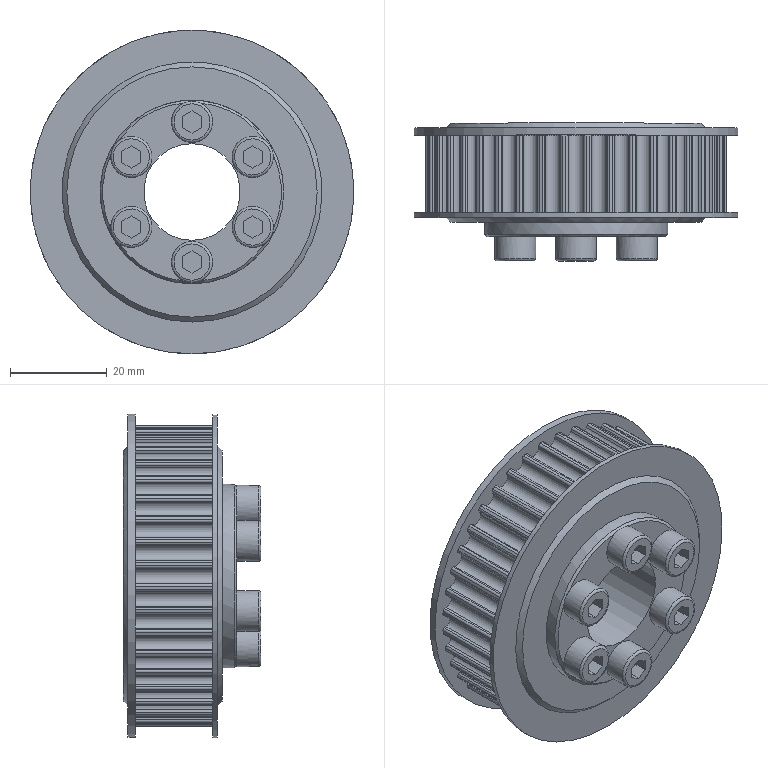Part | STEP file | YBQDJ-PD-4 | 1 solid | 338 faces | box 67 x 28.5 x 67 mm | volume 55543 mm3 | cylinder 176 | plane 147 | cone 9 | torus 6 | commonest cylinder face diameters 1 x80 3.12 x40 62.52 x40 4.2 x6 8.5 x6 67 x2